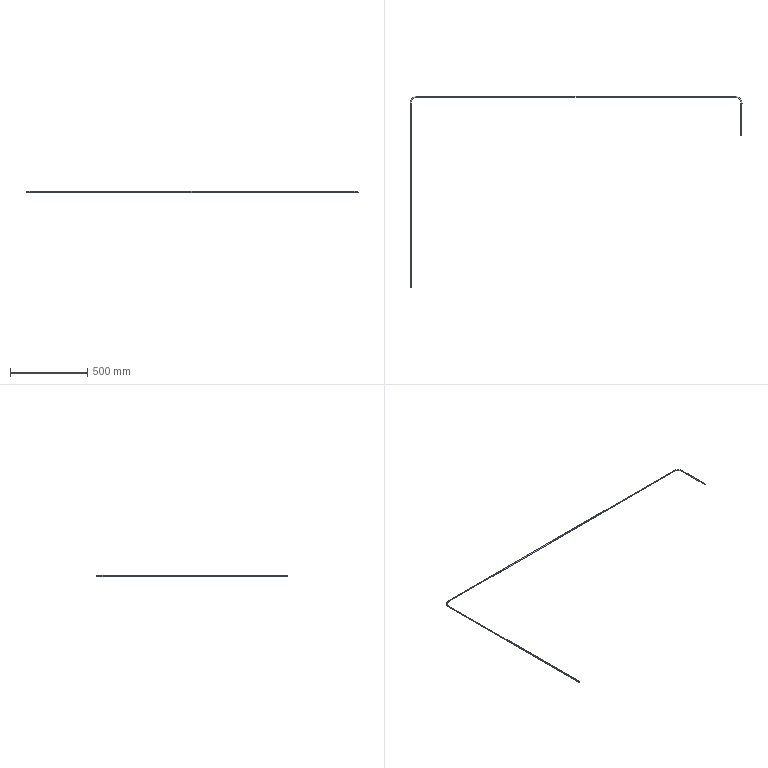Part | SolidWorks | features Sweep 1 | 1 solid | 12 faces | box 2149 x 1238 x 6.5 mm | volume 119159 mm3 | cylinder 6 | torus 4 | plane 2 | commonest cylinder face diameters 6.5 x6
STEP:
#1=CARTESIAN_POINT('',(2100.,1235.,-3.25));
#2=VERTEX_POINT('',#1);
#3=CARTESIAN_POINT('',(2100.,1238.25,0.));
#4=VERTEX_POINT('',#3);
#5=CARTESIAN_POINT('',(2100.,1235.,0.));
#6=DIRECTION('',(1.,0.,0.));
#7=DIRECTION('',(0.,0.,1.));
#8=AXIS2_PLACEMENT_3D('',#5,#6,#7);
#9=CIRCLE('',#8,3.25);
#10=EDGE_CURVE('',#2,#4,#9,.T.);
#11=ORIENTED_EDGE('',*,*,#10,.T.);
#12=CARTESIAN_POINT('',(2145.25,1193.,0.));
#13=VERTEX_POINT('',#12);
#14=CARTESIAN_POINT('',(2100.,1193.,0.));
#15=DIRECTION('',(0.,0.,-1.));
#16=DIRECTION('',(-1.,0.,0.));
#17=AXIS2_PLACEMENT_3D('',#14,#15,#16);
#18=CIRCLE('',#17,45.25);
#19=EDGE_CURVE('',#4,#13,#18,.T.);
#20=ORIENTED_EDGE('',*,*,#19,.T.);
#21=CARTESIAN_POINT('',(2142.,1193.,-3.25));
#22=VERTEX_POINT('',#21);
#23=CARTESIAN_POINT('',(2142.,1193.,0.));
#24=DIRECTION('',(0.,-1.,0.));
#25=DIRECTION('',(0.,0.,1.));
#26=AXIS2_PLACEMENT_3D('',#23,#24,#25);
#27=CIRCLE('',#26,3.25);
#28=EDGE_CURVE('',#22,#13,#27,.T.);
#29=ORIENTED_EDGE('',*,*,#28,.F.);
#30=CARTESIAN_POINT('',(2138.75,1193.,0.));
#31=VERTEX_POINT('',#30);
#32=CARTESIAN_POINT('',(2142.,1193.,0.));
#33=DIRECTION('',(0.,-1.,0.));
#34=DIRECTION('',(0.,0.,1.));
#35=AXIS2_PLACEMENT_3D('',#32,#33,#34);
#36=CIRCLE('',#35,3.25);
#37=EDGE_CURVE('',#31,#22,#36,.T.);
#38=ORIENTED_EDGE('',*,*,#37,.F.);
#39=CARTESIAN_POINT('',(2100.,1231.75,0.));
#40=VERTEX_POINT('',#39);
#41=CARTESIAN_POINT('',(2100.,1193.,0.));
#42=DIRECTION('',(0.,0.,-1.));
#43=DIRECTION('',(-1.,0.,0.));
#44=AXIS2_PLACEMENT_3D('',#41,#42,#43);
#45=CIRCLE('',#44,38.75);
#46=EDGE_CURVE('',#40,#31,#45,.T.);
#47=ORIENTED_EDGE('',*,*,#46,.F.);
#48=CARTESIAN_POINT('',(2100.,1235.,0.));
#49=DIRECTION('',(1.,0.,0.));
#50=DIRECTION('',(0.,0.,1.));
#51=AXIS2_PLACEMENT_3D('',#48,#49,#50);
#52=CIRCLE('',#51,3.25);
#53=EDGE_CURVE('',#40,#2,#52,.T.);
#54=ORIENTED_EDGE('',*,*,#53,.T.);
#55=EDGE_LOOP('',(#11,#20,#29,#38,#47,#54));
#56=FACE_OUTER_BOUND('',#55,.T.);
#57=CARTESIAN_POINT('',(2100.,1193.,0.));
#58=DIRECTION('',(0.,0.,-1.));
#59=DIRECTION('',(-1.,0.,0.));
#60=AXIS2_PLACEMENT_3D('',#57,#58,#59);
#61=TOROIDAL_SURFACE('',#60,42.,3.25);
#62=ADVANCED_FACE('',(#56),#61,.T.);
#63=CARTESIAN_POINT('',(0.,1193.,-3.25));
#64=VERTEX_POINT('',#63);
#65=CARTESIAN_POINT('',(-3.25,1193.,0.));
#66=VERTEX_POINT('',#65);
#67=CARTESIAN_POINT('',(0.,1193.,0.));
#68=DIRECTION('',(0.,1.,0.));
#69=DIRECTION('',(0.,0.,1.));
#70=AXIS2_PLACEMENT_3D('',#67,#68,#69);
#71=CIRCLE('',#70,3.25);
#72=EDGE_CURVE('',#64,#66,#71,.T.);
#73=ORIENTED_EDGE('',*,*,#72,.T.);
#74=CARTESIAN_POINT('',(42.,1238.25,0.));
#75=VERTEX_POINT('',#74);
#76=CARTESIAN_POINT('',(42.,1193.,0.));
#77=DIRECTION('',(0.,0.,-1.));
#78=DIRECTION('',(-1.,0.,0.));
#79=AXIS2_PLACEMENT_3D('',#76,#77,#78);
#80=CIRCLE('',#79,45.25);
#81=EDGE_CURVE('',#66,#75,#80,.T.);
#82=ORIENTED_EDGE('',*,*,#81,.T.);
#83=CARTESIAN_POINT('',(42.,1235.,-3.25));
#84=VERTEX_POINT('',#83);
#85=CARTESIAN_POINT('',(42.,1235.,0.));
#86=DIRECTION('',(1.,0.,0.));
#87=DIRECTION('',(0.,0.,1.));
#88=AXIS2_PLACEMENT_3D('',#85,#86,#87);
#89=CIRCLE('',#88,3.25);
#90=EDGE_CURVE('',#84,#75,#89,.T.);
#91=ORIENTED_EDGE('',*,*,#90,.F.);
#92=CARTESIAN_POINT('',(42.,1231.75,0.));
#93=VERTEX_POINT('',#92);
#94=CARTESIAN_POINT('',(42.,1235.,0.));
#95=DIRECTION('',(1.,0.,0.));
#96=DIRECTION('',(0.,0.,1.));
#97=AXIS2_PLACEMENT_3D('',#94,#95,#96);
#98=CIRCLE('',#97,3.25);
#99=EDGE_CURVE('',#93,#84,#98,.T.);
#100=ORIENTED_EDGE('',*,*,#99,.F.);
#101=CARTESIAN_POINT('',(3.25,1193.,0.));
#102=VERTEX_POINT('',#101);
#103=CARTESIAN_POINT('',(42.,1193.,0.));
#104=DIRECTION('',(0.,0.,-1.));
#105=DIRECTION('',(-1.,0.,0.));
#106=AXIS2_PLACEMENT_3D('',#103,#104,#105);
#107=CIRCLE('',#106,38.75);
#108=EDGE_CURVE('',#102,#93,#107,.T.);
#109=ORIENTED_EDGE('',*,*,#108,.F.);
#110=CARTESIAN_POINT('',(0.,1193.,0.));
#111=DIRECTION('',(0.,1.,0.));
#112=DIRECTION('',(0.,0.,1.));
#113=AXIS2_PLACEMENT_3D('',#110,#111,#112);
#114=CIRCLE('',#113,3.25);
#115=EDGE_CURVE('',#102,#64,#114,.T.);
#116=ORIENTED_EDGE('',*,*,#115,.T.);
#117=EDGE_LOOP('',(#73,#82,#91,#100,#109,#116));
#118=FACE_OUTER_BOUND('',#117,.T.);
#119=CARTESIAN_POINT('',(42.,1193.,0.));
#120=DIRECTION('',(0.,0.,-1.));
#121=DIRECTION('',(-1.,0.,0.));
#122=AXIS2_PLACEMENT_3D('',#119,#120,#121);
#123=TOROIDAL_SURFACE('',#122,42.,3.25);
#124=ADVANCED_FACE('',(#118),#123,.T.);
#125=ORIENTED_EDGE('',*,*,#28,.T.);
#126=CARTESIAN_POINT('',(2142.,1193.,3.25));
#127=VERTEX_POINT('',#126);
#128=CARTESIAN_POINT('',(2142.,1193.,0.));
#129=DIRECTION('',(0.,-1.,0.));
#130=DIRECTION('',(0.,0.,1.));
#131=AXIS2_PLACEMENT_3D('',#128,#129,#130);
#132=CIRCLE('',#131,3.25);
#133=EDGE_CURVE('',#13,#127,#132,.T.);
#134=ORIENTED_EDGE('',*,*,#133,.T.);
#135=CARTESIAN_POINT('',(2142.,985.,3.25));
#136=VERTEX_POINT('',#135);
#137=CARTESIAN_POINT('',(2142.,1193.,3.25));
#138=DIRECTION('',(0.,-1.,0.));
#139=VECTOR('',#138,1000.);
#140=LINE('',#137,#139);
#141=EDGE_CURVE('',#127,#136,#140,.T.);
#142=ORIENTED_EDGE('',*,*,#141,.T.);
#143=CARTESIAN_POINT('',(2142.,985.,-3.25));
#144=VERTEX_POINT('',#143);
#145=CARTESIAN_POINT('',(2142.,985.,0.));
#146=DIRECTION('',(0.,-1.,0.));
#147=DIRECTION('',(0.,0.,1.));
#148=AXIS2_PLACEMENT_3D('',#145,#146,#147);
#149=CIRCLE('',#148,3.25);
#150=EDGE_CURVE('',#144,#136,#149,.T.);
#151=ORIENTED_EDGE('',*,*,#150,.F.);
#152=CARTESIAN_POINT('',(2142.,1193.,-3.25));
#153=DIRECTION('',(0.,-1.,0.));
#154=VECTOR('',#153,1000.);
#155=LINE('',#152,#154);
#156=EDGE_CURVE('',#22,#144,#155,.T.);
#157=ORIENTED_EDGE('',*,*,#156,.F.);
#158=EDGE_LOOP('',(#125,#134,#142,#151,#157));
#159=FACE_OUTER_BOUND('',#158,.T.);
#160=CARTESIAN_POINT('',(2142.,1193.,0.));
#161=DIRECTION('',(0.,-1.,0.));
#162=DIRECTION('',(0.,0.,-1.));
#163=AXIS2_PLACEMENT_3D('',#160,#161,#162);
#164=CYLINDRICAL_SURFACE('',#163,3.25);
#165=ADVANCED_FACE('',(#159),#164,.T.);
#166=ORIENTED_EDGE('',*,*,#90,.T.);
#167=CARTESIAN_POINT('',(42.,1235.,3.25));
#168=VERTEX_POINT('',#167);
#169=CARTESIAN_POINT('',(42.,1235.,0.));
#170=DIRECTION('',(1.,0.,0.));
#171=DIRECTION('',(0.,0.,1.));
#172=AXIS2_PLACEMENT_3D('',#169,#170,#171);
#173=CIRCLE('',#172,3.25);
#174=EDGE_CURVE('',#75,#168,#173,.T.);
#175=ORIENTED_EDGE('',*,*,#174,.T.);
#176=CARTESIAN_POINT('',(2100.,1235.,3.25));
#177=VERTEX_POINT('',#176);
#178=CARTESIAN_POINT('',(42.,1235.,3.25));
#179=DIRECTION('',(1.,0.,0.));
#180=VECTOR('',#179,1000.);
#181=LINE('',#178,#180);
#182=EDGE_CURVE('',#168,#177,#181,.T.);
#183=ORIENTED_EDGE('',*,*,#182,.T.);
#184=CARTESIAN_POINT('',(2100.,1235.,0.));
#185=DIRECTION('',(1.,0.,0.));
#186=DIRECTION('',(0.,0.,1.));
#187=AXIS2_PLACEMENT_3D('',#184,#185,#186);
#188=CIRCLE('',#187,3.25);
#189=EDGE_CURVE('',#4,#177,#188,.T.);
#190=ORIENTED_EDGE('',*,*,#189,.F.);
#191=ORIENTED_EDGE('',*,*,#10,.F.);
#192=CARTESIAN_POINT('',(42.,1235.,-3.25));
#193=DIRECTION('',(1.,0.,0.));
#194=VECTOR('',#193,1000.);
#195=LINE('',#192,#194);
#196=EDGE_CURVE('',#84,#2,#195,.T.);
#197=ORIENTED_EDGE('',*,*,#196,.F.);
#198=EDGE_LOOP('',(#166,#175,#183,#190,#191,#197));
#199=FACE_OUTER_BOUND('',#198,.T.);
#200=CARTESIAN_POINT('',(42.,1235.,0.));
#201=DIRECTION('',(1.,0.,0.));
#202=DIRECTION('',(0.,0.,-1.));
#203=AXIS2_PLACEMENT_3D('',#200,#201,#202);
#204=CYLINDRICAL_SURFACE('',#203,3.25);
#205=ADVANCED_FACE('',(#199),#204,.T.);
#206=CARTESIAN_POINT('',(0.,0.,3.25));
#207=VERTEX_POINT('',#206);
#208=CARTESIAN_POINT('',(0.,0.,-3.25));
#209=VERTEX_POINT('',#208);
#210=CARTESIAN_POINT('',(0.,0.,0.));
#211=DIRECTION('',(0.,1.,0.));
#212=DIRECTION('',(0.,0.,1.));
#213=AXIS2_PLACEMENT_3D('',#210,#211,#212);
#214=CIRCLE('',#213,3.25);
#215=EDGE_CURVE('',#207,#209,#214,.T.);
#216=ORIENTED_EDGE('',*,*,#215,.T.);
#217=CARTESIAN_POINT('',(0.,0.,-3.25));
#218=DIRECTION('',(0.,1.,0.));
#219=VECTOR('',#218,1000.);
#220=LINE('',#217,#219);
#221=EDGE_CURVE('',#209,#64,#220,.T.);
#222=ORIENTED_EDGE('',*,*,#221,.T.);
#223=ORIENTED_EDGE('',*,*,#115,.F.);
#224=CARTESIAN_POINT('',(0.,1193.,3.25));
#225=VERTEX_POINT('',#224);
#226=CARTESIAN_POINT('',(0.,1193.,0.));
#227=DIRECTION('',(0.,1.,0.));
#228=DIRECTION('',(0.,0.,1.));
#229=AXIS2_PLACEMENT_3D('',#226,#227,#228);
#230=CIRCLE('',#229,3.25);
#231=EDGE_CURVE('',#225,#102,#230,.T.);
#232=ORIENTED_EDGE('',*,*,#231,.F.);
#233=CARTESIAN_POINT('',(0.,0.,3.25));
#234=DIRECTION('',(0.,1.,0.));
#235=VECTOR('',#234,1000.);
#236=LINE('',#233,#235);
#237=EDGE_CURVE('',#207,#225,#236,.T.);
#238=ORIENTED_EDGE('',*,*,#237,.F.);
#239=EDGE_LOOP('',(#216,#222,#223,#232,#238));
#240=FACE_OUTER_BOUND('',#239,.T.);
#241=CARTESIAN_POINT('',(0.,0.,0.));
#242=DIRECTION('',(0.,1.,0.));
#243=DIRECTION('',(0.,0.,1.));
#244=AXIS2_PLACEMENT_3D('',#241,#242,#243);
#245=CYLINDRICAL_SURFACE('',#244,3.25);
#246=ADVANCED_FACE('',(#240),#245,.T.);
#247=ORIENTED_EDGE('',*,*,#141,.F.);
#248=CARTESIAN_POINT('',(2142.,1193.,0.));
#249=DIRECTION('',(0.,-1.,0.));
#250=DIRECTION('',(0.,0.,1.));
#251=AXIS2_PLACEMENT_3D('',#248,#249,#250);
#252=CIRCLE('',#251,3.25);
#253=EDGE_CURVE('',#127,#31,#252,.T.);
#254=ORIENTED_EDGE('',*,*,#253,.T.);
#255=ORIENTED_EDGE('',*,*,#37,.T.);
#256=ORIENTED_EDGE('',*,*,#156,.T.);
#257=CARTESIAN_POINT('',(2142.,985.,0.));
#258=DIRECTION('',(0.,-1.,0.));
#259=DIRECTION('',(0.,0.,1.));
#260=AXIS2_PLACEMENT_3D('',#257,#258,#259);
#261=CIRCLE('',#260,3.25);
#262=EDGE_CURVE('',#136,#144,#261,.T.);
#263=ORIENTED_EDGE('',*,*,#262,.F.);
#264=EDGE_LOOP('',(#247,#254,#255,#256,#263));
#265=FACE_OUTER_BOUND('',#264,.T.);
#266=CARTESIAN_POINT('',(2142.,1193.,0.));
#267=DIRECTION('',(0.,-1.,0.));
#268=DIRECTION('',(0.,0.,-1.));
#269=AXIS2_PLACEMENT_3D('',#266,#267,#268);
#270=CYLINDRICAL_SURFACE('',#269,3.25);
#271=ADVANCED_FACE('',(#265),#270,.T.);
#272=ORIENTED_EDGE('',*,*,#19,.F.);
#273=ORIENTED_EDGE('',*,*,#189,.T.);
#274=CARTESIAN_POINT('',(2100.,1235.,0.));
#275=DIRECTION('',(1.,0.,0.));
#276=DIRECTION('',(0.,0.,1.));
#277=AXIS2_PLACEMENT_3D('',#274,#275,#276);
#278=CIRCLE('',#277,3.25);
#279=EDGE_CURVE('',#177,#40,#278,.T.);
#280=ORIENTED_EDGE('',*,*,#279,.T.);
#281=ORIENTED_EDGE('',*,*,#46,.T.);
#282=ORIENTED_EDGE('',*,*,#253,.F.);
#283=ORIENTED_EDGE('',*,*,#133,.F.);
#284=EDGE_LOOP('',(#272,#273,#280,#281,#282,#283));
#285=FACE_OUTER_BOUND('',#284,.T.);
#286=CARTESIAN_POINT('',(2100.,1193.,0.));
#287=DIRECTION('',(0.,0.,-1.));
#288=DIRECTION('',(-1.,0.,0.));
#289=AXIS2_PLACEMENT_3D('',#286,#287,#288);
#290=TOROIDAL_SURFACE('',#289,42.,3.25);
#291=ADVANCED_FACE('',(#285),#290,.T.);
#292=ORIENTED_EDGE('',*,*,#182,.F.);
#293=CARTESIAN_POINT('',(42.,1235.,0.));
#294=DIRECTION('',(1.,0.,0.));
#295=DIRECTION('',(0.,0.,1.));
#296=AXIS2_PLACEMENT_3D('',#293,#294,#295);
#297=CIRCLE('',#296,3.25);
#298=EDGE_CURVE('',#168,#93,#297,.T.);
#299=ORIENTED_EDGE('',*,*,#298,.T.);
#300=ORIENTED_EDGE('',*,*,#99,.T.);
#301=ORIENTED_EDGE('',*,*,#196,.T.);
#302=ORIENTED_EDGE('',*,*,#53,.F.);
#303=ORIENTED_EDGE('',*,*,#279,.F.);
#304=EDGE_LOOP('',(#292,#299,#300,#301,#302,#303));
#305=FACE_OUTER_BOUND('',#304,.T.);
#306=CARTESIAN_POINT('',(42.,1235.,0.));
#307=DIRECTION('',(1.,0.,0.));
#308=DIRECTION('',(0.,0.,-1.));
#309=AXIS2_PLACEMENT_3D('',#306,#307,#308);
#310=CYLINDRICAL_SURFACE('',#309,3.25);
#311=ADVANCED_FACE('',(#305),#310,.T.);
#312=ORIENTED_EDGE('',*,*,#81,.F.);
#313=CARTESIAN_POINT('',(0.,1193.,0.));
#314=DIRECTION('',(0.,1.,0.));
#315=DIRECTION('',(0.,0.,1.));
#316=AXIS2_PLACEMENT_3D('',#313,#314,#315);
#317=CIRCLE('',#316,3.25);
#318=EDGE_CURVE('',#66,#225,#317,.T.);
#319=ORIENTED_EDGE('',*,*,#318,.T.);
#320=ORIENTED_EDGE('',*,*,#231,.T.);
#321=ORIENTED_EDGE('',*,*,#108,.T.);
#322=ORIENTED_EDGE('',*,*,#298,.F.);
#323=ORIENTED_EDGE('',*,*,#174,.F.);
#324=EDGE_LOOP('',(#312,#319,#320,#321,#322,#323));
#325=FACE_OUTER_BOUND('',#324,.T.);
#326=CARTESIAN_POINT('',(42.,1193.,0.));
#327=DIRECTION('',(0.,0.,-1.));
#328=DIRECTION('',(-1.,0.,0.));
#329=AXIS2_PLACEMENT_3D('',#326,#327,#328);
#330=TOROIDAL_SURFACE('',#329,42.,3.25);
#331=ADVANCED_FACE('',(#325),#330,.T.);
#332=ORIENTED_EDGE('',*,*,#221,.F.);
#333=CARTESIAN_POINT('',(0.,0.,0.));
#334=DIRECTION('',(0.,1.,0.));
#335=DIRECTION('',(0.,0.,1.));
#336=AXIS2_PLACEMENT_3D('',#333,#334,#335);
#337=CIRCLE('',#336,3.25);
#338=EDGE_CURVE('',#209,#207,#337,.T.);
#339=ORIENTED_EDGE('',*,*,#338,.T.);
#340=ORIENTED_EDGE('',*,*,#237,.T.);
#341=ORIENTED_EDGE('',*,*,#318,.F.);
#342=ORIENTED_EDGE('',*,*,#72,.F.);
#343=EDGE_LOOP('',(#332,#339,#340,#341,#342));
#344=FACE_OUTER_BOUND('',#343,.T.);
#345=CARTESIAN_POINT('',(0.,0.,0.));
#346=DIRECTION('',(0.,1.,0.));
#347=DIRECTION('',(0.,0.,1.));
#348=AXIS2_PLACEMENT_3D('',#345,#346,#347);
#349=CYLINDRICAL_SURFACE('',#348,3.25);
#350=ADVANCED_FACE('',(#344),#349,.T.);
#351=ORIENTED_EDGE('',*,*,#150,.T.);
#352=ORIENTED_EDGE('',*,*,#262,.T.);
#353=EDGE_LOOP('',(#351,#352));
#354=FACE_OUTER_BOUND('',#353,.T.);
#355=CARTESIAN_POINT('',(2142.,985.,0.));
#356=DIRECTION('',(0.,-1.,0.));
#357=DIRECTION('',(0.,0.,1.));
#358=AXIS2_PLACEMENT_3D('',#355,#356,#357);
#359=PLANE('',#358);
#360=ADVANCED_FACE('',(#354),#359,.T.);
#361=ORIENTED_EDGE('',*,*,#215,.F.);
#362=ORIENTED_EDGE('',*,*,#338,.F.);
#363=EDGE_LOOP('',(#361,#362));
#364=FACE_OUTER_BOUND('',#363,.T.);
#365=CARTESIAN_POINT('',(0.,0.,0.));
#366=DIRECTION('',(0.,1.,0.));
#367=DIRECTION('',(0.,0.,1.));
#368=AXIS2_PLACEMENT_3D('',#365,#366,#367);
#369=PLANE('',#368);
#370=ADVANCED_FACE('',(#364),#369,.F.);
#371=CLOSED_SHELL('',(#62,#124,#165,#205,#246,#271,#291,#311,#331,#350,#360,#370));
#372=MANIFOLD_SOLID_BREP('',#371);
#373=CARTESIAN_POINT('',(0.,0.,0.));
#374=DIRECTION('',(0.,0.,1.));
#375=DIRECTION('',(1.,0.,0.));
#376=AXIS2_PLACEMENT_3D('',#373,#374,#375);
#377=(LENGTH_UNIT()NAMED_UNIT(*)SI_UNIT(.MILLI.,.METRE.));
#378=UNCERTAINTY_MEASURE_WITH_UNIT(LENGTH_MEASURE(0.00001),#377,'','');
#379=(NAMED_UNIT(*)PLANE_ANGLE_UNIT()SI_UNIT($,.RADIAN.));
#380=(NAMED_UNIT(*)SI_UNIT($,.STERADIAN.)SOLID_ANGLE_UNIT());
#381=(GEOMETRIC_REPRESENTATION_CONTEXT(3)GLOBAL_UNCERTAINTY_ASSIGNED_CONTEXT((#378))GLOBAL_UNIT_ASSIGNED_CONTEXT((#377,#379,#380))REPRESENTATION_CONTEXT('',''));
#382=ADVANCED_BREP_SHAPE_REPRESENTATION('',(#372,#376),#381);